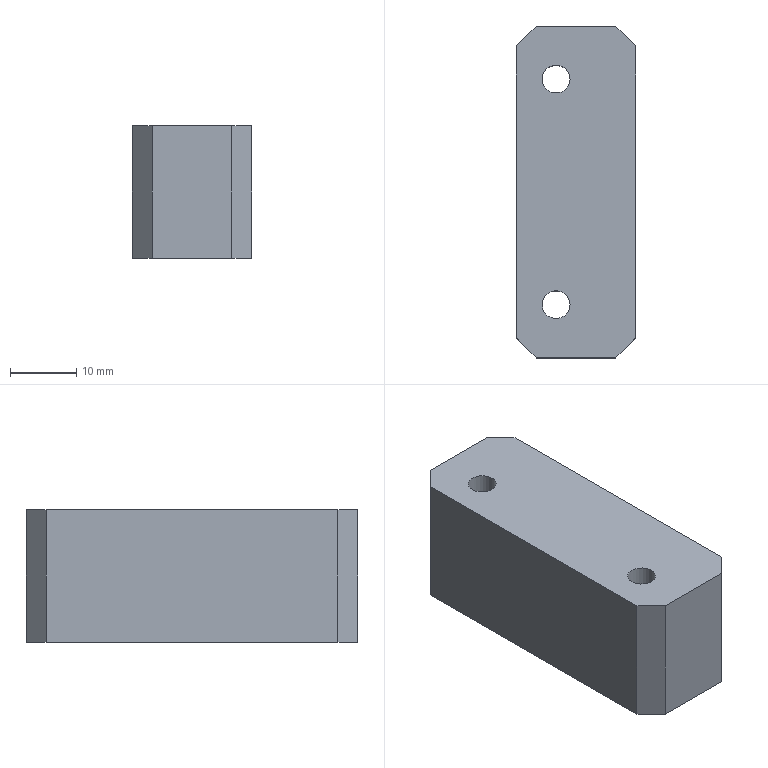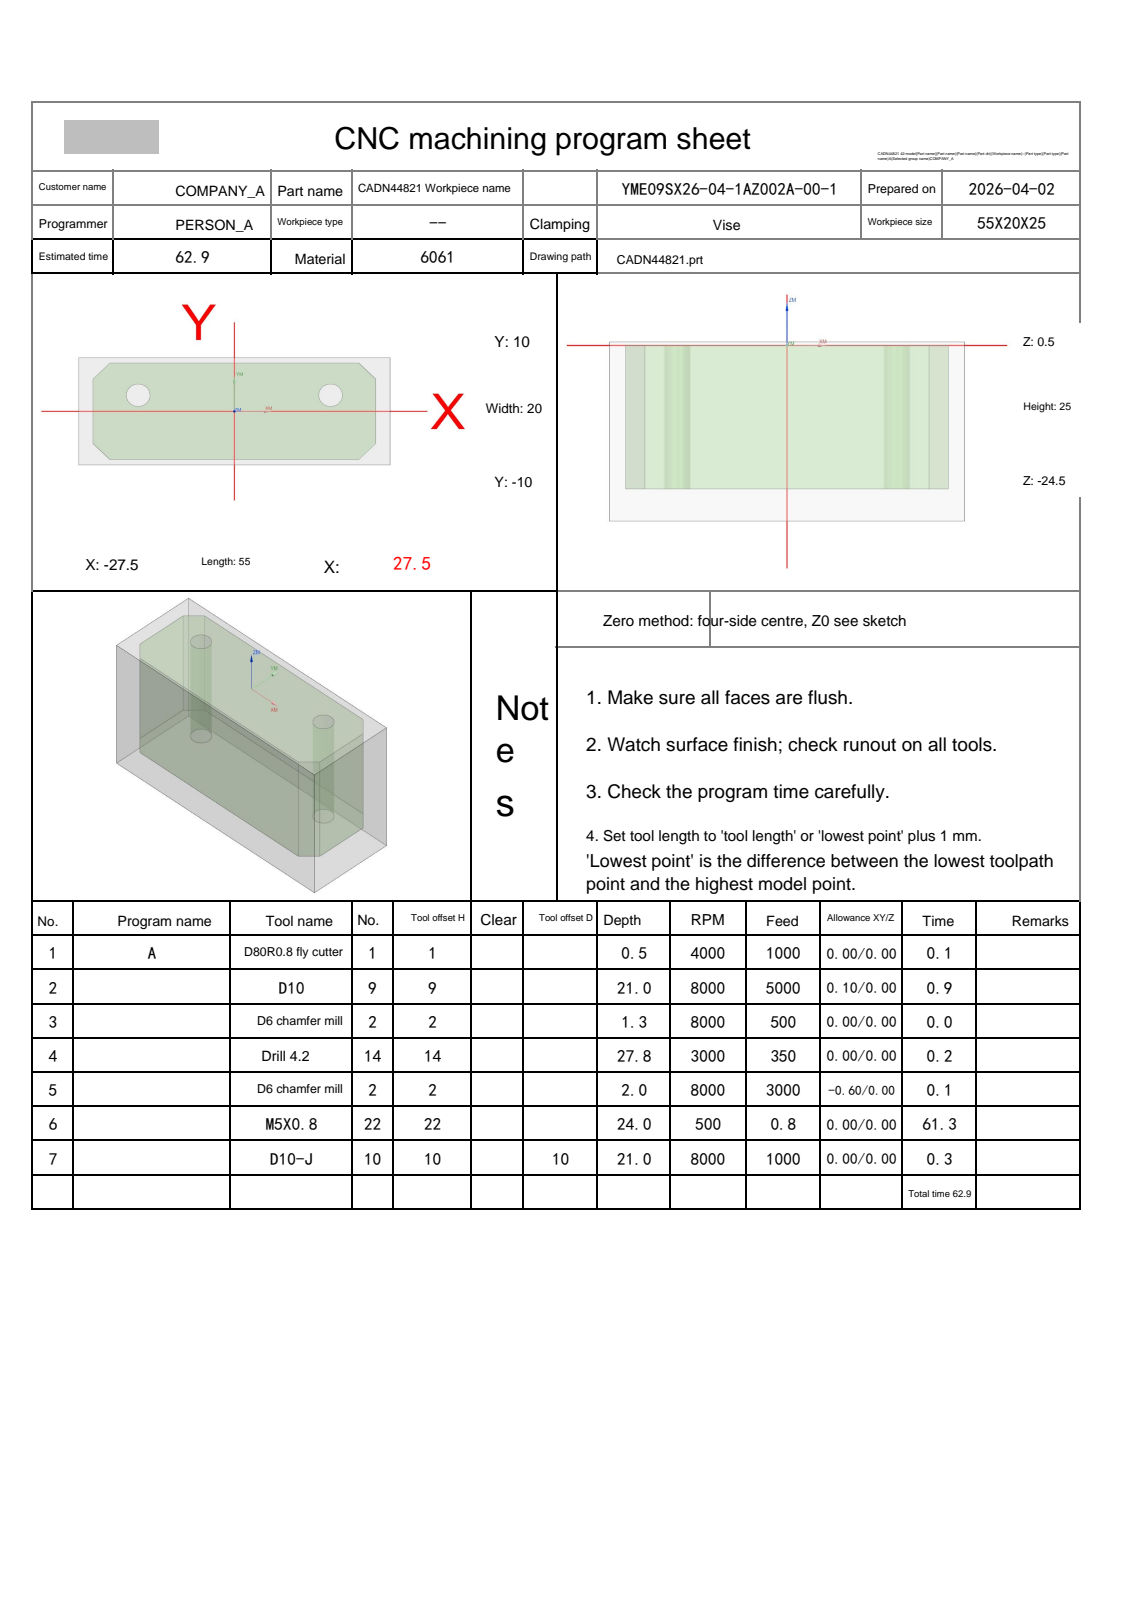NC program | NX | posted by the shop | part box 18 x 50 x 20 mm
Whole program:
%
O0001
(Machine time: 123.13 MIN)
(===Total Tool:6===)
(T1=D80R0.8 fly cutter D=80.  R=0.8  D-  H01 Z=-0.   )
(T9=D10     D=10.  R=0.   D-  H09 Z=-20.5 )
(T2=D6 chamfer mill   D=6.   R=0.   D-  H02 Z=-1.5  )
(T14=drill 4.2  D=4.2  DR_a=118 D-  H14 Z=-27.26)
(T22=M5X0.8 D=4.2  DR_a=180 D-  H22 Z=-23.5 )
(T10=D10-J  D=10.  R=0.   D10 H10 Z=-20.5 )
G80 G90 G17 G49 G40
G91 G28 Z0
M01
N1 T01 M06
(D80R0.8 fly cutter  D=80. R=0.8 H=01 ce=0.00 di=0.00)
G00 G90 G54 X-70. Y0.0 M03 S4000
G43 H01 Z20.
M08
Z2.
G01 Z0.0 F1000.
X-65.
X65.
X70.
Z2.
G00 Z20.
G91 G28 Z0.0
M05
M09
G91 G28 Z0.0
M01
N2 T09 M06
(D10  D=10. R=0. H=09 ce=0.10 di=0.00)
G00 G90 G54 X0.0 Y-14.1 M03 S8000
G43 H09 Z20.
M08
Z.5
G01 X-22. Z.394 F5000.
G02 X-25.606 Y-12.606 Z.374 I0.0 J5.1
G01 X-28.606 Y-9.606 Z.354
G02 X-30.1 Y-6. Z.335 I3.606 J3.606
G01 Y6. Z.277
G02 X-28.606 Y9.606 Z.257 I5.1 J0.0
G01 X-25.606 Y12.606 Z.237
G02 X-22. Y14.1 Z.217 I3.606 J-3.606
G01 X22. Z.005
G02 X25.606 Y12.606 Z-.015 I0.0 J-5.1
G01 X28.606 Y9.606 Z-.035
G02 X30.1 Y6. Z-.054 I-3.606 J-3.606
G01 Y-6. Z-.112
G02 X28.606 Y-9.606 Z-.132 I-5.1 J0.0
G01 X25.606 Y-12.606 Z-.152
G02 X22. Y-14.1 Z-.172 I-3.606 J3.606
G01 X-22. Z-.384
G02 X-25.606 Y-12.606 Z-.403 I0.0 J5.1
G01 X-28.606 Y-9.606 Z-.424
G02 X-30.1 Y-6. Z-.443 I3.606 J3.606
G01 Y6. Z-.501
G02 X-28.606 Y9.606 Z-.521 I5.1 J0.0
G01 X-25.606 Y12.606 Z-.541
G02 X-22. Y14.1 Z-.56 I3.606 J-3.606
G01 X22. Z-.773
G02 X25.606 Y12.606 Z-.792 I0.0 J-5.1
G01 X28.606 Y9.606 Z-.813
G02 X30.1 Y6. Z-.832 I-3.606 J-3.606
G01 Y-6. Z-.89
G02 X28.606 Y-9.606 Z-.909 I-5.1 J0.0
G01 X25.606 Y-12.606 Z-.93
G02 X22. Y-14.1 Z-.949 I-3.606 J3.606
G01 X-22. Z-1.162
G02 X-25.606 Y-12.606 Z-1.181 I0.0 J5.1
G01 X-28.606 Y-9.606 Z-1.202
G02 X-30.1 Y-6. Z-1.221 I3.606 J3.606
G01 Y6. Z-1.279
G02 X-28.606 Y9.606 Z-1.298 I5.1 J0.0
G01 X-25.606 Y12.606 Z-1.319
G02 X-22. Y14.1 Z-1.338 I3.606 J-3.606
G01 X22. Z-1.551
G02 X25.606 Y12.606 Z-1.57 I0.0 J-5.1
G01 X28.606 Y9.606 Z-1.591
G02 X30.1 Y6. Z-1.61 I-3.606 J-3.606
G01 Y-6. Z-1.668
G02 X28.606 Y-9.606 Z-1.687 I-5.1 J0.0
G01 X25.606 Y-12.606 Z-1.708
G02 X22. Y-14.1 Z-1.727 I-3.606 J3.606
G01 X-22. Z-1.94
G02 X-25.606 Y-12.606 Z-1.959 I0.0 J5.1
G01 X-28.606 Y-9.606 Z-1.979
G02 X-30.1 Y-6. Z-1.999 I3.606 J3.606
G01 Y6. Z-2.057
G02 X-28.606 Y9.606 Z-2.076 I5.1 J0.0
G01 X-25.606 Y12.606 Z-2.097
G02 X-22. Y14.1 Z-2.116 I3.606 J-3.606
G01 X22. Z-2.328
G02 X25.606 Y12.606 Z-2.348 I0.0 J-5.1
G01 X28.606 Y9.606 Z-2.368
G02 X30.1 Y6. Z-2.388 I-3.606 J-3.606
G01 Y-6. Z-2.446
G02 X28.606 Y-9.606 Z-2.465 I-5.1 J0.0
G01 X25.606 Y-12.606 Z-2.485
G02 X22. Y-14.1 Z-2.505 I-3.606 J3.606
G01 X-22. Z-2.717
G02 X-25.606 Y-12.606 Z-2.737 I0.0 J5.1
G01 X-28.606 Y-9.606 Z-2.757
G02 X-30.1 Y-6. Z-2.777 I3.606 J3.606
G01 Y6. Z-2.835
G02 X-28.606 Y9.606 Z-2.854 I5.1 J0.0
G01 X-25.606 Y12.606 Z-2.874
G02 X-22. Y14.1 Z-2.894 I3.606 J-3.606
G01 X22. Z-3.106
G02 X25.606 Y12.606 Z-3.126 I0.0 J-5.1
G01 X28.606 Y9.606 Z-3.146
G02 X30.1 Y6. Z-3.165 I-3.606 J-3.606
G01 Y-6. Z-3.223
G02 X28.606 Y-9.606 Z-3.243 I-5.1 J0.0
G01 X25.606 Y-12.606 Z-3.263
G02 X22. Y-14.1 Z-3.283 I-3.606 J3.606
G01 X-22. Z-3.495
G02 X-25.606 Y-12.606 Z-3.515 I0.0 J5.1
G01 X-28.606 Y-9.606 Z-3.535
G02 X-30.1 Y-6. Z-3.554 I3.606 J3.606
G01 Y6. Z-3.612
G02 X-28.606 Y9.606 Z-3.632 I5.1 J0.0
G01 X-25.606 Y12.606 Z-3.652
G02 X-22. Y14.1 Z-3.672 I3.606 J-3.606
G01 X22. Z-3.884
G02 X25.606 Y12.606 Z-3.903 I0.0 J-5.1
G01 X28.606 Y9.606 Z-3.924
G02 X30.1 Y6. Z-3.943 I-3.606 J-3.606
G01 Y-6. Z-4.001
G02 X28.606 Y-9.606 Z-4.021 I-5.1 J0.0
G01 X25.606 Y-12.606 Z-4.041
G02 X22. Y-14.1 Z-4.06 I-3.606 J3.606
G01 X-22. Z-4.273
G02 X-25.606 Y-12.606 Z-4.292 I0.0 J5.1
G01 X-28.606 Y-9.606 Z-4.313
G02 X-30.1 Y-6. Z-4.332 I3.606 J3.606
G01 Y6. Z-4.39
G02 X-28.606 Y9.606 Z-4.409 I5.1 J0.0
G01 X-25.606 Y12.606 Z-4.43
G02 X-22. Y14.1 Z-4.449 I3.606 J-3.606
G01 X22. Z-4.662
G02 X25.606 Y12.606 Z-4.681 I0.0 J-5.1
G01 X28.606 Y9.606 Z-4.702
G02 X30.1 Y6. Z-4.721 I-3.606 J-3.606
G01 Y-6. Z-4.779
G02 X28.606 Y-9.606 Z-4.798 I-5.1 J0.0
G01 X25.606 Y-12.606 Z-4.819
G02 X22. Y-14.1 Z-4.838 I-3.606 J3.606
G01 X-22. Z-5.051
G02 X-25.606 Y-12.606 Z-5.07 I0.0 J5.1
G01 X-28.606 Y-9.606 Z-5.091
G02 X-30.1 Y-6. Z-5.11 I3.606 J3.606
G01 Y6. Z-5.168
G02 X-28.606 Y9.606 Z-5.187 I5.1 J0.0
G01 X-25.606 Y12.606 Z-5.208
G02 X-22. Y14.1 Z-5.227 I3.606 J-3.606
G01 X22. Z-5.44
G02 X25.606 Y12.606 Z-5.459 I0.0 J-5.1
G01 X28.606 Y9.606 Z-5.479
G02 X30.1 Y6. Z-5.499 I-3.606 J-3.606
G01 Y-6. Z-5.557
G02 X28.606 Y-9.606 Z-5.576 I-5.1 J0.0
G01 X25.606 Y-12.606 Z-5.597
G02 X22. Y-14.1 Z-5.616 I-3.606 J3.606
G01 X-22. Z-5.828
G02 X-25.606 Y-12.606 Z-5.848 I0.0 J5.1
G01 X-28.606 Y-9.606 Z-5.868
G02 X-30.1 Y-6. Z-5.888 I3.606 J3.606
G01 Y6. Z-5.946
G02 X-28.606 Y9.606 Z-5.965 I5.1 J0.0
G01 X-25.606 Y12.606 Z-5.985
G02 X-22. Y14.1 Z-6.005 I3.606 J-3.606
G01 X22. Z-6.217
G02 X25.606 Y12.606 Z-6.237 I0.0 J-5.1
G01 X28.606 Y9.606 Z-6.257
G02 X30.1 Y6. Z-6.277 I-3.606 J-3.606
G01 Y-6. Z-6.335
G02 X28.606 Y-9.606 Z-6.354 I-5.1 J0.0
G01 X25.606 Y-12.606 Z-6.374
G02 X22. Y-14.1 Z-6.394 I-3.606 J3.606
G01 X-22. Z-6.606
G02 X-25.606 Y-12.606 Z-6.626 I0.0 J5.1
G01 X-28.606 Y-9.606 Z-6.646
G02 X-30.1 Y-6. Z-6.665 I3.606 J3.606
G01 Y6. Z-6.723
G02 X-28.606 Y9.606 Z-6.743 I5.1 J0.0
G01 X-25.606 Y12.606 Z-6.763
G02 X-22. Y14.1 Z-6.783 I3.606 J-3.606
G01 X22. Z-6.995
G02 X25.606 Y12.606 Z-7.015 I0.0 J-5.1
G01 X28.606 Y9.606 Z-7.035
G02 X30.1 Y6. Z-7.054 I-3.606 J-3.606
G01 Y-6. Z-7.112
G02 X28.606 Y-9.606 Z-7.132 I-5.1 J0.0
G01 X25.606 Y-12.606 Z-7.152
G02 X22. Y-14.1 Z-7.172 I-3.606 J3.606
G01 X-22. Z-7.384
G02 X-25.606 Y-12.606 Z-7.403 I0.0 J5.1
G01 X-28.606 Y-9.606 Z-7.424
G02 X-30.1 Y-6. Z-7.443 I3.606 J3.606
G01 Y6. Z-7.501
G02 X-28.606 Y9.606 Z-7.521 I5.1 J0.0
G01 X-25.606 Y12.606 Z-7.541
G02 X-22. Y14.1 Z-7.56 I3.606 J-3.606
G01 X22. Z-7.773
G02 X25.606 Y12.606 Z-7.792 I0.0 J-5.1
G01 X28.606 Y9.606 Z-7.813
G02 X30.1 Y6. Z-7.832 I-3.606 J-3.606
G01 Y-6. Z-7.89
G02 X28.606 Y-9.606 Z-7.909 I-5.1 J0.0
G01 X25.606 Y-12.606 Z-7.93
G02 X22. Y-14.1 Z-7.949 I-3.606 J3.606
G01 X-22. Z-8.162
G02 X-25.606 Y-12.606 Z-8.181 I0.0 J5.1
G01 X-28.606 Y-9.606 Z-8.202
G02 X-30.1 Y-6. Z-8.221 I3.606 J3.606
G01 Y6. Z-8.279
G02 X-28.606 Y9.606 Z-8.298 I5.1 J0.0
G01 X-25.606 Y12.606 Z-8.319
G02 X-22. Y14.1 Z-8.338 I3.606 J-3.606
G01 X22. Z-8.551
G02 X25.606 Y12.606 Z-8.57 I0.0 J-5.1
G01 X28.606 Y9.606 Z-8.591
G02 X30.1 Y6. Z-8.61 I-3.606 J-3.606
G01 Y-6. Z-8.668
G02 X28.606 Y-9.606 Z-8.687 I-5.1 J0.0
G01 X25.606 Y-12.606 Z-8.708
G02 X22. Y-14.1 Z-8.727 I-3.606 J3.606
G01 X-22. Z-8.94
G02 X-25.606 Y-12.606 Z-8.959 I0.0 J5.1
G01 X-28.606 Y-9.606 Z-8.979
G02 X-30.1 Y-6. Z-8.999 I3.606 J3.606
G01 Y6. Z-9.057
G02 X-28.606 Y9.606 Z-9.076 I5.1 J0.0
G01 X-25.606 Y12.606 Z-9.097
G02 X-22. Y14.1 Z-9.116 I3.606 J-3.606
G01 X22. Z-9.328
G02 X25.606 Y12.606 Z-9.348 I0.0 J-5.1
G01 X28.606 Y9.606 Z-9.368
G02 X30.1 Y6. Z-9.388 I-3.606 J-3.606
G01 Y-6. Z-9.446
G02 X28.606 Y-9.606 Z-9.465 I-5.1 J0.0
G01 X25.606 Y-12.606 Z-9.485
G02 X22. Y-14.1 Z-9.505 I-3.606 J3.606
G01 X-22. Z-9.717
G02 X-25.606 Y-12.606 Z-9.737 I0.0 J5.1
G01 X-28.606 Y-9.606 Z-9.757
G02 X-30.1 Y-6. Z-9.777 I3.606 J3.606
G01 Y6. Z-9.835
G02 X-28.606 Y9.606 Z-9.854 I5.1 J0.0
G01 X-25.606 Y12.606 Z-9.874
G02 X-22. Y14.1 Z-9.894 I3.606 J-3.606
G01 X22. Z-10.106
G02 X25.606 Y12.606 Z-10.126 I0.0 J-5.1
G01 X28.606 Y9.606 Z-10.146
G02 X30.1 Y6. Z-10.165 I-3.606 J-3.606
G01 Y-6. Z-10.223
G02 X28.606 Y-9.606 Z-10.243 I-5.1 J0.0
G01 X25.606 Y-12.606 Z-10.263
G02 X22. Y-14.1 Z-10.283 I-3.606 J3.606
G01 X-22. Z-10.495
G02 X-25.606 Y-12.606 Z-10.515 I0.0 J5.1
G01 X-28.606 Y-9.606 Z-10.535
G02 X-30.1 Y-6. Z-10.554 I3.606 J3.606
G01 Y6. Z-10.612
G02 X-28.606 Y9.606 Z-10.632 I5.1 J0.0
G01 X-25.606 Y12.606 Z-10.652
G02 X-22. Y14.1 Z-10.672 I3.606 J-3.606
G01 X22. Z-10.884
G02 X25.606 Y12.606 Z-10.903 I0.0 J-5.1
G01 X28.606 Y9.606 Z-10.924
G02 X30.1 Y6. Z-10.943 I-3.606 J-3.606
G01 Y-6. Z-11.001
G02 X28.606 Y-9.606 Z-11.021 I-5.1 J0.0
G01 X25.606 Y-12.606 Z-11.041
G02 X22. Y-14.1 Z-11.06 I-3.606 J3.606
G01 X-22. Z-11.273
G02 X-25.606 Y-12.606 Z-11.292 I0.0 J5.1
G01 X-28.606 Y-9.606 Z-11.313
G02 X-30.1 Y-6. Z-11.332 I3.606 J3.606
G01 Y6. Z-11.39
G02 X-28.606 Y9.606 Z-11.409 I5.1 J0.0
G01 X-25.606 Y12.606 Z-11.43
G02 X-22. Y14.1 Z-11.449 I3.606 J-3.606
G01 X22. Z-11.662
G02 X25.606 Y12.606 Z-11.681 I0.0 J-5.1
G01 X28.606 Y9.606 Z-11.702
G02 X30.1 Y6. Z-11.721 I-3.606 J-3.606
G01 Y-6. Z-11.779
G02 X28.606 Y-9.606 Z-11.798 I-5.1 J0.0
G01 X25.606 Y-12.606 Z-11.819
G02 X22. Y-14.1 Z-11.838 I-3.606 J3.606
G01 X-22. Z-12.051
G02 X-25.606 Y-12.606 Z-12.07 I0.0 J5.1
G01 X-28.606 Y-9.606 Z-12.091
G02 X-30.1 Y-6. Z-12.11 I3.606 J3.606
G01 Y6. Z-12.168
G02 X-28.606 Y9.606 Z-12.187 I5.1 J0.0
G01 X-25.606 Y12.606 Z-12.208
G02 X-22. Y14.1 Z-12.227 I3.606 J-3.606
G01 X22. Z-12.44
G02 X25.606 Y12.606 Z-12.459 I0.0 J-5.1
G01 X28.606 Y9.606 Z-12.479
G02 X30.1 Y6. Z-12.499 I-3.606 J-3.606
G01 Y-6. Z-12.557
G02 X28.606 Y-9.606 Z-12.576 I-5.1 J0.0
G01 X25.606 Y-12.606 Z-12.597
G02 X22. Y-14.1 Z-12.616 I-3.606 J3.606
G01 X-22. Z-12.828
G02 X-25.606 Y-12.606 Z-12.848 I0.0 J5.1
G01 X-28.606 Y-9.606 Z-12.868
G02 X-30.1 Y-6. Z-12.888 I3.606 J3.606
G01 Y6. Z-12.946
G02 X-28.606 Y9.606 Z-12.965 I5.1 J0.0
G01 X-25.606 Y12.606 Z-12.985
G02 X-22. Y14.1 Z-13.005 I3.606 J-3.606
G01 X22. Z-13.217
G02 X25.606 Y12.606 Z-13.237 I0.0 J-5.1
G01 X28.606 Y9.606 Z-13.257
G02 X30.1 Y6. Z-13.277 I-3.606 J-3.606
G01 Y-6. Z-13.335
G02 X28.606 Y-9.606 Z-13.354 I-5.1 J0.0
G01 X25.606 Y-12.606 Z-13.374
G02 X22. Y-14.1 Z-13.394 I-3.606 J3.606
G01 X-22. Z-13.606
G02 X-25.606 Y-12.606 Z-13.626 I0.0 J5.1
G01 X-28.606 Y-9.606 Z-13.646
G02 X-30.1 Y-6. Z-13.665 I3.606 J3.606
G01 Y6. Z-13.723
G02 X-28.606 Y9.606 Z-13.743 I5.1 J0.0
G01 X-25.606 Y12.606 Z-13.763
G02 X-22. Y14.1 Z-13.783 I3.606 J-3.606
G01 X22. Z-13.995
G02 X25.606 Y12.606 Z-14.015 I0.0 J-5.1
G01 X28.606 Y9.606 Z-14.035
G02 X30.1 Y6. Z-14.054 I-3.606 J-3.606
G01 Y-6. Z-14.112
G02 X28.606 Y-9.606 Z-14.132 I-5.1 J0.0
G01 X25.606 Y-12.606 Z-14.152
G02 X22. Y-14.1 Z-14.172 I-3.606 J3.606
G01 X-22. Z-14.384
G02 X-25.606 Y-12.606 Z-14.403 I0.0 J5.1
G01 X-28.606 Y-9.606 Z-14.424
G02 X-30.1 Y-6. Z-14.443 I3.606 J3.606
G01 Y6. Z-14.501
G02 X-28.606 Y9.606 Z-14.521 I5.1 J0.0
G01 X-25.606 Y12.606 Z-14.541
G02 X-22. Y14.1 Z-14.56 I3.606 J-3.606
G01 X22. Z-14.773
G02 X25.606 Y12.606 Z-14.792 I0.0 J-5.1
G01 X28.606 Y9.606 Z-14.813
G02 X30.1 Y6. Z-14.832 I-3.606 J-3.606
G01 Y-6. Z-14.89
G02 X28.606 Y-9.606 Z-14.909 I-5.1 J0.0
G01 X25.606 Y-12.606 Z-14.93
G02 X22. Y-14.1 Z-14.949 I-3.606 J3.606
G01 X-22. Z-15.162
G02 X-25.606 Y-12.606 Z-15.181 I0.0 J5.1
G01 X-28.606 Y-9.606 Z-15.202
G02 X-30.1 Y-6. Z-15.221 I3.606 J3.606
G01 Y6. Z-15.279
G02 X-28.606 Y9.606 Z-15.298 I5.1 J0.0
G01 X-25.606 Y12.606 Z-15.319
G02 X-22. Y14.1 Z-15.338 I3.606 J-3.606
G01 X22. Z-15.551
G02 X25.606 Y12.606 Z-15.57 I0.0 J-5.1
G01 X28.606 Y9.606 Z-15.591
G02 X30.1 Y6. Z-15.61 I-3.606 J-3.606
G01 Y-6. Z-15.668
G02 X28.606 Y-9.606 Z-15.687 I-5.1 J0.0
G01 X25.606 Y-12.606 Z-15.708
G02 X22. Y-14.1 Z-15.727 I-3.606 J3.606
G01 X-22. Z-15.94
G02 X-25.606 Y-12.606 Z-15.959 I0.0 J5.1
G01 X-28.606 Y-9.606 Z-15.979
G02 X-30.1 Y-6. Z-15.999 I3.606 J3.606
G01 Y6. Z-16.057
G02 X-28.606 Y9.606 Z-16.076 I5.1 J0.0
G01 X-25.606 Y12.606 Z-16.097
G02 X-22. Y14.1 Z-16.116 I3.606 J-3.606
G01 X22. Z-16.328
G02 X25.606 Y12.606 Z-16.348 I0.0 J-5.1
G01 X28.606 Y9.606 Z-16.368
G02 X30.1 Y6. Z-16.388 I-3.606 J-3.606
G01 Y-6. Z-16.446
G02 X28.606 Y-9.606 Z-16.465 I-5.1 J0.0
G01 X25.606 Y-12.606 Z-16.485
G02 X22. Y-14.1 Z-16.505 I-3.606 J3.606
G01 X-22. Z-16.717
G02 X-25.606 Y-12.606 Z-16.737 I0.0 J5.1
G01 X-28.606 Y-9.606 Z-16.757
G02 X-30.1 Y-6. Z-16.777 I3.606 J3.606
G01 Y6. Z-16.835
G02 X-28.606 Y9.606 Z-16.854 I5.1 J0.0
G01 X-25.606 Y12.606 Z-16.874
G02 X-22. Y14.1 Z-16.894 I3.606 J-3.606
G01 X22. Z-17.106
G02 X25.606 Y12.606 Z-17.126 I0.0 J-5.1
G01 X28.606 Y9.606 Z-17.146
G02 X30.1 Y6. Z-17.165 I-3.606 J-3.606
G01 Y-6. Z-17.223
G02 X28.606 Y-9.606 Z-17.243 I-5.1 J0.0
G01 X25.606 Y-12.606 Z-17.263
G02 X22. Y-14.1 Z-17.283 I-3.606 J3.606
G01 X-22. Z-17.495
G02 X-25.606 Y-12.606 Z-17.515 I0.0 J5.1
G01 X-28.606 Y-9.606 Z-17.535
G02 X-30.1 Y-6. Z-17.554 I3.606 J3.606
G01 Y6. Z-17.612
G02 X-28.606 Y9.606 Z-17.632 I5.1 J0.0
G01 X-25.606 Y12.606 Z-17.652
G02 X-22. Y14.1 Z-17.672 I3.606 J-3.606
G01 X22. Z-17.884
G02 X25.606 Y12.606 Z-17.903 I0.0 J-5.1
G01 X28.606 Y9.606 Z-17.924
G02 X30.1 Y6. Z-17.943 I-3.606 J-3.606
G01 Y-6. Z-18.001
G02 X28.606 Y-9.606 Z-18.021 I-5.1 J0.0
G01 X25.606 Y-12.606 Z-18.041
G02 X22. Y-14.1 Z-18.06 I-3.606 J3.606
G01 X-22. Z-18.273
G02 X-25.606 Y-12.606 Z-18.292 I0.0 J5.1
G01 X-28.606 Y-9.606 Z-18.313
G02 X-30.1 Y-6. Z-18.332 I3.606 J3.606
G01 Y6. Z-18.39
G02 X-28.606 Y9.606 Z-18.409 I5.1 J0.0
G01 X-25.606 Y12.606 Z-18.43
G02 X-22. Y14.1 Z-18.449 I3.606 J-3.606
G01 X22. Z-18.662
G02 X25.606 Y12.606 Z-18.681 I0.0 J-5.1
G01 X28.606 Y9.606 Z-18.702
G02 X30.1 Y6. Z-18.721 I-3.606 J-3.606
G01 Y-6. Z-18.779
G02 X28.606 Y-9.606 Z-18.798 I-5.1 J0.0
G01 X25.606 Y-12.606 Z-18.819
G02 X22. Y-14.1 Z-18.838 I-3.606 J3.606
G01 X-22. Z-19.051
G02 X-25.606 Y-12.606 Z-19.07 I0.0 J5.1
G01 X-28.606 Y-9.606 Z-19.091
G02 X-30.1 Y-6. Z-19.11 I3.606 J3.606
G01 Y6. Z-19.168
G02 X-28.606 Y9.606 Z-19.187 I5.1 J0.0
G01 X-25.606 Y12.606 Z-19.208
G02 X-22. Y14.1 Z-19.227 I3.606 J-3.606
G01 X22. Z-19.44
G02 X25.606 Y12.606 Z-19.459 I0.0 J-5.1
G01 X28.606 Y9.606 Z-19.479
G02 X30.1 Y6. Z-19.499 I-3.606 J-3.606
G01 Y-6. Z-19.557
G02 X28.606 Y-9.606 Z-19.576 I-5.1 J0.0
G01 X25.606 Y-12.606 Z-19.597
G02 X22. Y-14.1 Z-19.616 I-3.606 J3.606
G01 X-22. Z-19.828
G02 X-25.606 Y-12.606 Z-19.848 I0.0 J5.1
G01 X-28.606 Y-9.606 Z-19.868
G02 X-30.1 Y-6. Z-19.888 I3.606 J3.606
G01 Y6. Z-19.946
G02 X-28.606 Y9.606 Z-19.965 I5.1 J0.0
G01 X-25.606 Y12.606 Z-19.985
G02 X-22. Y14.1 Z-20.005 I3.606 J-3.606
G01 X22. Z-20.217
G02 X25.606 Y12.606 Z-20.237 I0.0 J-5.1
G01 X28.606 Y9.606 Z-20.257
G02 X30.1 Y6. Z-20.277 I-3.606 J-3.606
G01 Y-6. Z-20.335
G02 X28.606 Y-9.606 Z-20.354 I-5.1 J0.0
G01 X25.606 Y-12.606 Z-20.374
G02 X22. Y-14.1 Z-20.394 I-3.606 J3.606
G01 X0.0 Z-20.5
X-22.
G02 X-25.606 Y-12.606 I0.0 J5.1
G01 X-28.606 Y-9.606
G02 X-30.1 Y-6. I3.606 J3.606
G01 Y6.
G02 X-28.606 Y9.606 I5.1 J0.0
G01 X-25.606 Y12.606
G02 X-22. Y14.1 I3.606 J-3.606
G01 X22.
G02 X25.606 Y12.606 I0.0 J-5.1
G01 X28.606 Y9.606
G02 X30.1 Y6. I-3.606 J-3.606
G01 Y-6.
G02 X28.606 Y-9.606 I-5.1 J0.0
G01 X25.606 Y-12.606
G02 X22. Y-14.1 I-3.606 J3.606
G01 X0.0
X-.5
Z-19.5
G00 Z20.
G91 G28 Z0.0
M05
M09
G91 G28 Z0.0
M01
N3 T02 M06
(D6 chamfer mill  D=6. R=0. H=02 ce=0.00 di=0.00)
G00 G90 G54 X-17. Y3. M03 S8000
G43 H02 Z20.
M08
G98 G81 X-17. Y3. Z-.8 R1. F500.
X17.
G80
G00 Z20.
G91 G28 Z0.0
M05
M09
G91 G28 Z0.0
M01
N4 T14 M06
(Drill 4.2 D=4.2 DR_a=118 H=14)
G00 G90 G54 X-17. Y3. M03 S3000
G43 H14 Z20.
M08
G98 G83 X-17. Y3. Z-27.262 R1. F350. Q3.
X17.
G80
G00 Z20.
G91 G28 Z0.0
M05
M09
G91 G28 Z0.0
M01
N5 T02 M06
(D6 chamfer mill  D=6. R=0. H=02 ce=0.00 di=0.00)
G00 G90 G54 X-.25 Y11.128 M03 S8000
G43 H02 Z20.
M08
Z2.099
G01 Z-1.5 F3000.
G03 X-.33 Y10.828 I.52 J-.3
X-.03 Y10.308 I.6 J0.0
G01 X0.0 Y10.3
X22.
X22.254 Y10.275
X22.497 Y10.201
X22.722 Y10.081
X22.919 Y9.919
X25.919 Y6.919
X26.081 Y6.722
X26.201 Y6.497
X26.275 Y6.254
X26.3 Y6.
Y-6.
X26.275 Y-6.254
X26.201 Y-6.497
X26.081 Y-6.722
X25.919 Y-6.919
X22.919 Y-9.919
X22.722 Y-10.081
X22.497 Y-10.201
X22.254 Y-10.275
X22. Y-10.3
X-22.
X-22.254 Y-10.275
X-22.497 Y-10.201
X-22.722 Y-10.081
X-22.919 Y-9.919
X-25.919 Y-6.919
X-26.081 Y-6.722
X-26.201 Y-6.497
X-26.275 Y-6.254
X-26.3 Y-6.
Y6.
X-26.275 Y6.254
X-26.201 Y6.497
X-26.081 Y6.722
X-25.919 Y6.919
X-22.919 Y9.919
X-22.722 Y10.081
X-22.498 Y10.201
X-22.254 Y10.275
X-22. Y10.3
X0.0
X.03 Y10.308
G03 X.33 Y10.828 I-.3 J.52
X.25 Y11.128 I-.6 J0.0
G01 Z2.099
G00 Z20.
G00 G90 X-16.306 Y3.093 M03 S8000
Z20.
Z-.5
G01 Z-1. F500.
X-15.5 Y3.2
G03 X-17. Y4.7 I-1.5 J0.0
X-18.7 Y3. I0.0 J-1.7
X-17. Y1.3 I1.7 J0.0
X-15.3 Y3. I0.0 J1.7
X-17. Y4.7 I-1.7 J0.0
X-18.5 Y3.2 I0.0 J-1.5
G01 X-17.694 Y3.093
Z-.5
G00 Z20.
X17.694
Z-.5
G01 Z-1.
X18.5 Y3.2
G03 X17. Y4.7 I-1.5 J0.0
X15.3 Y3. I0.0 J-1.7
X17. Y1.3 I1.7 J0.0
X18.7 Y3. I0.0 J1.7
X17. Y4.7 I-1.7 J0.0
X15.5 Y3.2 I0.0 J-1.5
G01 X16.306 Y3.093
Z-.5
G00 Z20.
G91 G28 Z0.0
M05
M09
G91 G28 Z0.0
M01
N6 T22 M06
(M5X0.8 D=4.2 DR_a=180 H=22)
G00 G90 G54 X-17. Y3. M03 S500
G43 H22 Z20.
M08
G95
G98 G84 X-17. Y3. Z-23.5 R1. F.8 Q3.
X17.
G80
G94
G00 Z20.
G91 G28 Z0.0
M05
M09
G91 G28 Z0.0
M01
N7 T10 M06
(D10-J  D=10. R=0. H=10 ce=0.00 di=0.00)
G00 G90 G54 X23.013 Y-15.116 M03 S8000
G43 H10 Z20.
M08
Z-9.75
G01 Z-10.25 F1000.
G41 D10
X22.997 Y-14.917
G03 X22. Y-14. I-.997 J-.083
G01 X-22.
G02 X-25.536 Y-12.536 I0.0 J5.
G01 X-28.536 Y-9.536
G02 X-30. Y-6. I3.536 J3.536
G01 Y6.
G02 X-28.536 Y9.536 I5. J0.0
G01 X-25.536 Y12.536
G02 X-22. Y14. I3.536 J-3.536
G01 X22.
G02 X25.536 Y12.536 I0.0 J-5.
G01 X28.536 Y9.536
G02 X30. Y6. I-3.536 J-3.536
G01 Y-6.
G02 X28.536 Y-9.536 I-5. J0.0
G01 X25.536 Y-12.536
G02 X22. Y-14. I-3.536 J3.536
G01 X21.5
G03 X20.5 Y-15. I0.0 J-1.
G01 G40 Y-15.2
Z-9.75
G00 Z20.
X23.013 Y-15.116
Z-20.
G01 Z-20.5
G41 D10
X22.997 Y-14.917
G03 X22. Y-14. I-.997 J-.083
G01 X-22.
G02 X-25.536 Y-12.536 I0.0 J5.
G01 X-28.536 Y-9.536
G02 X-30. Y-6. I3.536 J3.536
G01 Y6.
G02 X-28.536 Y9.536 I5. J0.0
G01 X-25.536 Y12.536
G02 X-22. Y14. I3.536 J-3.536
G01 X22.
G02 X25.536 Y12.536 I0.0 J-5.
G01 X28.536 Y9.536
G02 X30. Y6. I-3.536 J-3.536
G01 Y-6.
G02 X28.536 Y-9.536 I-5. J0.0
G01 X25.536 Y-12.536
G02 X22. Y-14. I-3.536 J3.536
G01 X21.5
G03 X20.5 Y-15. I0.0 J-1.
G01 G40 Y-15.2
Z-20.
G00 Z20.
M05
M09
G91 G28 Z0.0
G91 G28 Y0.0
M30
%